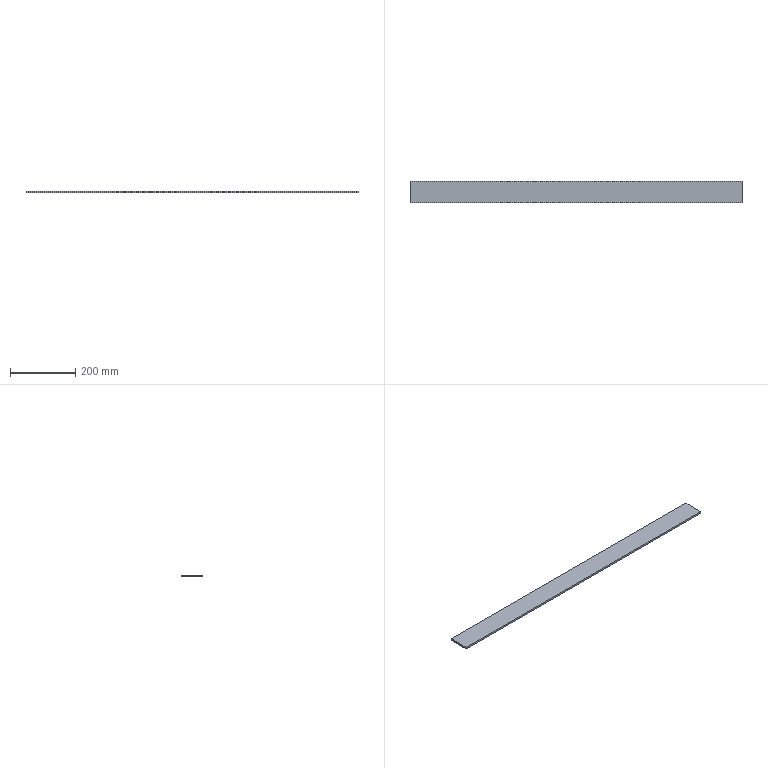Part | STEP file | 04-Support plate | 1 solid | 6 faces | box 1020 x 65 x 6 mm | volume 397800 mm3 | plane 6
STEP:
#1=CARTESIAN_POINT('',(0.,0.,0.));
#2=DIRECTION('',(0.,0.,1.));
#3=DIRECTION('',(1.,0.,0.));
#4=AXIS2_PLACEMENT_3D('',#1,#2,#3);
#5=CARTESIAN_POINT('',(0.,0.,0.));
#6=VERTEX_POINT('',#5);
#7=CARTESIAN_POINT('',(0.,-65.,0.));
#8=VERTEX_POINT('',#7);
#9=CARTESIAN_POINT('',(0.,0.,0.));
#10=DIRECTION('',(0.,-1.,0.));
#11=VECTOR('',#10,1.);
#12=LINE('',#9,#11);
#13=CARTESIAN_POINT('',(0.,0.,6.));
#14=DIRECTION('',(1.,0.,0.));
#15=DIRECTION('',(0.,1.,0.));
#16=AXIS2_PLACEMENT_3D('',#13,#14,#15);
#17=PLANE('',#16);
#18=CARTESIAN_POINT('',(0.,-6.));
#19=DIRECTION('',(-1.,0.));
#20=VECTOR('',#19,1.);
#21=LINE('',#18,#20);
#22=(GEOMETRIC_REPRESENTATION_CONTEXT(2)PARAMETRIC_REPRESENTATION_CONTEXT()REPRESENTATION_CONTEXT('',''));
#23=DEFINITIONAL_REPRESENTATION('',(#21),#22);
#24=PCURVE('',#17,#23);
#25=CARTESIAN_POINT('',(0.,0.,0.));
#26=DIRECTION('',(0.,0.,1.));
#27=DIRECTION('',(1.,0.,0.));
#28=AXIS2_PLACEMENT_3D('',#25,#26,#27);
#29=PLANE('',#28);
#30=CARTESIAN_POINT('',(0.,0.));
#31=DIRECTION('',(0.,-1.));
#32=VECTOR('',#31,1.);
#33=LINE('',#30,#32);
#34=(GEOMETRIC_REPRESENTATION_CONTEXT(2)PARAMETRIC_REPRESENTATION_CONTEXT()REPRESENTATION_CONTEXT('',''));
#35=DEFINITIONAL_REPRESENTATION('',(#33),#34);
#36=PCURVE('',#29,#35);
#37=SURFACE_CURVE('',#12,(#24,#36),.PCURVE_S1.);
#38=EDGE_CURVE('',#6,#8,#37,.T.);
#39=ORIENTED_EDGE('',*,*,#38,.T.);
#40=CARTESIAN_POINT('',(0.,-65.,6.));
#41=VERTEX_POINT('',#40);
#42=CARTESIAN_POINT('',(0.,-65.,6.));
#43=DIRECTION('',(0.,0.,-1.));
#44=VECTOR('',#43,1.);
#45=LINE('',#42,#44);
#46=CARTESIAN_POINT('',(-65.,0.));
#47=DIRECTION('',(0.,-1.));
#48=VECTOR('',#47,1.);
#49=LINE('',#46,#48);
#50=(GEOMETRIC_REPRESENTATION_CONTEXT(2)PARAMETRIC_REPRESENTATION_CONTEXT()REPRESENTATION_CONTEXT('',''));
#51=DEFINITIONAL_REPRESENTATION('',(#49),#50);
#52=PCURVE('',#17,#51);
#53=CARTESIAN_POINT('',(0.,-65.,6.));
#54=DIRECTION('',(0.,1.,0.));
#55=DIRECTION('',(0.,0.,1.));
#56=AXIS2_PLACEMENT_3D('',#53,#54,#55);
#57=PLANE('',#56);
#58=CARTESIAN_POINT('',(0.,0.));
#59=DIRECTION('',(-1.,0.));
#60=VECTOR('',#59,1.);
#61=LINE('',#58,#60);
#62=(GEOMETRIC_REPRESENTATION_CONTEXT(2)PARAMETRIC_REPRESENTATION_CONTEXT()REPRESENTATION_CONTEXT('',''));
#63=DEFINITIONAL_REPRESENTATION('',(#61),#62);
#64=PCURVE('',#57,#63);
#65=SURFACE_CURVE('',#45,(#52,#64),.PCURVE_S1.);
#66=EDGE_CURVE('',#41,#8,#65,.T.);
#67=ORIENTED_EDGE('',*,*,#66,.F.);
#68=CARTESIAN_POINT('',(0.,0.,6.));
#69=VERTEX_POINT('',#68);
#70=CARTESIAN_POINT('',(0.,0.,6.));
#71=DIRECTION('',(0.,-1.,0.));
#72=VECTOR('',#71,1.);
#73=LINE('',#70,#72);
#74=CARTESIAN_POINT('',(0.,0.));
#75=DIRECTION('',(-1.,0.));
#76=VECTOR('',#75,1.);
#77=LINE('',#74,#76);
#78=(GEOMETRIC_REPRESENTATION_CONTEXT(2)PARAMETRIC_REPRESENTATION_CONTEXT()REPRESENTATION_CONTEXT('',''));
#79=DEFINITIONAL_REPRESENTATION('',(#77),#78);
#80=PCURVE('',#17,#79);
#81=CARTESIAN_POINT('',(0.,0.,6.));
#82=DIRECTION('',(0.,0.,1.));
#83=DIRECTION('',(1.,0.,0.));
#84=AXIS2_PLACEMENT_3D('',#81,#82,#83);
#85=PLANE('',#84);
#86=CARTESIAN_POINT('',(0.,0.));
#87=DIRECTION('',(0.,-1.));
#88=VECTOR('',#87,1.);
#89=LINE('',#86,#88);
#90=(GEOMETRIC_REPRESENTATION_CONTEXT(2)PARAMETRIC_REPRESENTATION_CONTEXT()REPRESENTATION_CONTEXT('',''));
#91=DEFINITIONAL_REPRESENTATION('',(#89),#90);
#92=PCURVE('',#85,#91);
#93=SURFACE_CURVE('',#73,(#80,#92),.PCURVE_S1.);
#94=EDGE_CURVE('',#69,#41,#93,.T.);
#95=ORIENTED_EDGE('',*,*,#94,.F.);
#96=CARTESIAN_POINT('',(0.,0.,6.));
#97=DIRECTION('',(0.,0.,-1.));
#98=VECTOR('',#97,1.);
#99=LINE('',#96,#98);
#100=CARTESIAN_POINT('',(0.,0.));
#101=DIRECTION('',(0.,-1.));
#102=VECTOR('',#101,1.);
#103=LINE('',#100,#102);
#104=(GEOMETRIC_REPRESENTATION_CONTEXT(2)PARAMETRIC_REPRESENTATION_CONTEXT()REPRESENTATION_CONTEXT('',''));
#105=DEFINITIONAL_REPRESENTATION('',(#103),#104);
#106=PCURVE('',#17,#105);
#107=CARTESIAN_POINT('',(0.,0.,6.));
#108=DIRECTION('',(0.,-1.,0.));
#109=DIRECTION('',(0.,0.,-1.));
#110=AXIS2_PLACEMENT_3D('',#107,#108,#109);
#111=PLANE('',#110);
#112=CARTESIAN_POINT('',(0.,0.));
#113=DIRECTION('',(1.,0.));
#114=VECTOR('',#113,1.);
#115=LINE('',#112,#114);
#116=(GEOMETRIC_REPRESENTATION_CONTEXT(2)PARAMETRIC_REPRESENTATION_CONTEXT()REPRESENTATION_CONTEXT('',''));
#117=DEFINITIONAL_REPRESENTATION('',(#115),#116);
#118=PCURVE('',#111,#117);
#119=SURFACE_CURVE('',#99,(#106,#118),.PCURVE_S1.);
#120=EDGE_CURVE('',#69,#6,#119,.T.);
#121=ORIENTED_EDGE('',*,*,#120,.T.);
#122=EDGE_LOOP('',(#39,#67,#95,#121));
#123=FACE_BOUND('',#122,.T.);
#124=ADVANCED_FACE('',(#123),#17,.F.);
#125=CARTESIAN_POINT('',(1020.,-65.,0.));
#126=VERTEX_POINT('',#125);
#127=CARTESIAN_POINT('',(0.,-65.,0.));
#128=DIRECTION('',(1.,0.,0.));
#129=VECTOR('',#128,1.);
#130=LINE('',#127,#129);
#131=CARTESIAN_POINT('',(-6.,0.));
#132=DIRECTION('',(0.,1.));
#133=VECTOR('',#132,1.);
#134=LINE('',#131,#133);
#135=(GEOMETRIC_REPRESENTATION_CONTEXT(2)PARAMETRIC_REPRESENTATION_CONTEXT()REPRESENTATION_CONTEXT('',''));
#136=DEFINITIONAL_REPRESENTATION('',(#134),#135);
#137=PCURVE('',#57,#136);
#138=CARTESIAN_POINT('',(0.,-65.));
#139=DIRECTION('',(1.,0.));
#140=VECTOR('',#139,1.);
#141=LINE('',#138,#140);
#142=(GEOMETRIC_REPRESENTATION_CONTEXT(2)PARAMETRIC_REPRESENTATION_CONTEXT()REPRESENTATION_CONTEXT('',''));
#143=DEFINITIONAL_REPRESENTATION('',(#141),#142);
#144=PCURVE('',#29,#143);
#145=SURFACE_CURVE('',#130,(#137,#144),.PCURVE_S1.);
#146=EDGE_CURVE('',#8,#126,#145,.T.);
#147=ORIENTED_EDGE('',*,*,#146,.T.);
#148=CARTESIAN_POINT('',(1020.,-65.,6.));
#149=VERTEX_POINT('',#148);
#150=CARTESIAN_POINT('',(1020.,-65.,6.));
#151=DIRECTION('',(0.,0.,-1.));
#152=VECTOR('',#151,1.);
#153=LINE('',#150,#152);
#154=CARTESIAN_POINT('',(0.,1020.));
#155=DIRECTION('',(-1.,0.));
#156=VECTOR('',#155,1.);
#157=LINE('',#154,#156);
#158=(GEOMETRIC_REPRESENTATION_CONTEXT(2)PARAMETRIC_REPRESENTATION_CONTEXT()REPRESENTATION_CONTEXT('',''));
#159=DEFINITIONAL_REPRESENTATION('',(#157),#158);
#160=PCURVE('',#57,#159);
#161=CARTESIAN_POINT('',(1020.,0.,6.));
#162=DIRECTION('',(-1.,0.,0.));
#163=DIRECTION('',(0.,0.,1.));
#164=AXIS2_PLACEMENT_3D('',#161,#162,#163);
#165=PLANE('',#164);
#166=CARTESIAN_POINT('',(0.,-65.));
#167=DIRECTION('',(-1.,0.));
#168=VECTOR('',#167,1.);
#169=LINE('',#166,#168);
#170=(GEOMETRIC_REPRESENTATION_CONTEXT(2)PARAMETRIC_REPRESENTATION_CONTEXT()REPRESENTATION_CONTEXT('',''));
#171=DEFINITIONAL_REPRESENTATION('',(#169),#170);
#172=PCURVE('',#165,#171);
#173=SURFACE_CURVE('',#153,(#160,#172),.PCURVE_S1.);
#174=EDGE_CURVE('',#149,#126,#173,.T.);
#175=ORIENTED_EDGE('',*,*,#174,.F.);
#176=CARTESIAN_POINT('',(0.,-65.,6.));
#177=DIRECTION('',(1.,0.,0.));
#178=VECTOR('',#177,1.);
#179=LINE('',#176,#178);
#180=CARTESIAN_POINT('',(0.,0.));
#181=DIRECTION('',(0.,1.));
#182=VECTOR('',#181,1.);
#183=LINE('',#180,#182);
#184=(GEOMETRIC_REPRESENTATION_CONTEXT(2)PARAMETRIC_REPRESENTATION_CONTEXT()REPRESENTATION_CONTEXT('',''));
#185=DEFINITIONAL_REPRESENTATION('',(#183),#184);
#186=PCURVE('',#57,#185);
#187=CARTESIAN_POINT('',(0.,-65.));
#188=DIRECTION('',(1.,0.));
#189=VECTOR('',#188,1.);
#190=LINE('',#187,#189);
#191=(GEOMETRIC_REPRESENTATION_CONTEXT(2)PARAMETRIC_REPRESENTATION_CONTEXT()REPRESENTATION_CONTEXT('',''));
#192=DEFINITIONAL_REPRESENTATION('',(#190),#191);
#193=PCURVE('',#85,#192);
#194=SURFACE_CURVE('',#179,(#186,#193),.PCURVE_S1.);
#195=EDGE_CURVE('',#41,#149,#194,.T.);
#196=ORIENTED_EDGE('',*,*,#195,.F.);
#197=ORIENTED_EDGE('',*,*,#66,.T.);
#198=EDGE_LOOP('',(#147,#175,#196,#197));
#199=FACE_BOUND('',#198,.T.);
#200=ADVANCED_FACE('',(#199),#57,.F.);
#201=CARTESIAN_POINT('',(1020.,0.,0.));
#202=VERTEX_POINT('',#201);
#203=CARTESIAN_POINT('',(1020.,0.,0.));
#204=DIRECTION('',(0.,1.,0.));
#205=VECTOR('',#204,1.);
#206=LINE('',#203,#205);
#207=CARTESIAN_POINT('',(-6.,0.));
#208=DIRECTION('',(0.,1.));
#209=VECTOR('',#208,1.);
#210=LINE('',#207,#209);
#211=(GEOMETRIC_REPRESENTATION_CONTEXT(2)PARAMETRIC_REPRESENTATION_CONTEXT()REPRESENTATION_CONTEXT('',''));
#212=DEFINITIONAL_REPRESENTATION('',(#210),#211);
#213=PCURVE('',#165,#212);
#214=CARTESIAN_POINT('',(1020.,0.));
#215=DIRECTION('',(0.,1.));
#216=VECTOR('',#215,1.);
#217=LINE('',#214,#216);
#218=(GEOMETRIC_REPRESENTATION_CONTEXT(2)PARAMETRIC_REPRESENTATION_CONTEXT()REPRESENTATION_CONTEXT('',''));
#219=DEFINITIONAL_REPRESENTATION('',(#217),#218);
#220=PCURVE('',#29,#219);
#221=SURFACE_CURVE('',#206,(#213,#220),.PCURVE_S1.);
#222=EDGE_CURVE('',#126,#202,#221,.T.);
#223=ORIENTED_EDGE('',*,*,#222,.T.);
#224=CARTESIAN_POINT('',(1020.,0.,6.));
#225=VERTEX_POINT('',#224);
#226=CARTESIAN_POINT('',(1020.,0.,6.));
#227=DIRECTION('',(0.,0.,-1.));
#228=VECTOR('',#227,1.);
#229=LINE('',#226,#228);
#230=CARTESIAN_POINT('',(0.,0.));
#231=DIRECTION('',(-1.,0.));
#232=VECTOR('',#231,1.);
#233=LINE('',#230,#232);
#234=(GEOMETRIC_REPRESENTATION_CONTEXT(2)PARAMETRIC_REPRESENTATION_CONTEXT()REPRESENTATION_CONTEXT('',''));
#235=DEFINITIONAL_REPRESENTATION('',(#233),#234);
#236=PCURVE('',#165,#235);
#237=CARTESIAN_POINT('',(0.,1020.));
#238=DIRECTION('',(1.,0.));
#239=VECTOR('',#238,1.);
#240=LINE('',#237,#239);
#241=(GEOMETRIC_REPRESENTATION_CONTEXT(2)PARAMETRIC_REPRESENTATION_CONTEXT()REPRESENTATION_CONTEXT('',''));
#242=DEFINITIONAL_REPRESENTATION('',(#240),#241);
#243=PCURVE('',#111,#242);
#244=SURFACE_CURVE('',#229,(#236,#243),.PCURVE_S1.);
#245=EDGE_CURVE('',#225,#202,#244,.T.);
#246=ORIENTED_EDGE('',*,*,#245,.F.);
#247=CARTESIAN_POINT('',(1020.,0.,6.));
#248=DIRECTION('',(0.,1.,0.));
#249=VECTOR('',#248,1.);
#250=LINE('',#247,#249);
#251=CARTESIAN_POINT('',(0.,0.));
#252=DIRECTION('',(0.,1.));
#253=VECTOR('',#252,1.);
#254=LINE('',#251,#253);
#255=(GEOMETRIC_REPRESENTATION_CONTEXT(2)PARAMETRIC_REPRESENTATION_CONTEXT()REPRESENTATION_CONTEXT('',''));
#256=DEFINITIONAL_REPRESENTATION('',(#254),#255);
#257=PCURVE('',#165,#256);
#258=CARTESIAN_POINT('',(1020.,0.));
#259=DIRECTION('',(0.,1.));
#260=VECTOR('',#259,1.);
#261=LINE('',#258,#260);
#262=(GEOMETRIC_REPRESENTATION_CONTEXT(2)PARAMETRIC_REPRESENTATION_CONTEXT()REPRESENTATION_CONTEXT('',''));
#263=DEFINITIONAL_REPRESENTATION('',(#261),#262);
#264=PCURVE('',#85,#263);
#265=SURFACE_CURVE('',#250,(#257,#264),.PCURVE_S1.);
#266=EDGE_CURVE('',#149,#225,#265,.T.);
#267=ORIENTED_EDGE('',*,*,#266,.F.);
#268=ORIENTED_EDGE('',*,*,#174,.T.);
#269=EDGE_LOOP('',(#223,#246,#267,#268));
#270=FACE_BOUND('',#269,.T.);
#271=ADVANCED_FACE('',(#270),#165,.F.);
#272=CARTESIAN_POINT('',(0.,0.,0.));
#273=DIRECTION('',(-1.,0.,0.));
#274=VECTOR('',#273,1.);
#275=LINE('',#272,#274);
#276=CARTESIAN_POINT('',(6.,0.));
#277=DIRECTION('',(0.,-1.));
#278=VECTOR('',#277,1.);
#279=LINE('',#276,#278);
#280=(GEOMETRIC_REPRESENTATION_CONTEXT(2)PARAMETRIC_REPRESENTATION_CONTEXT()REPRESENTATION_CONTEXT('',''));
#281=DEFINITIONAL_REPRESENTATION('',(#279),#280);
#282=PCURVE('',#111,#281);
#283=CARTESIAN_POINT('',(0.,0.));
#284=DIRECTION('',(-1.,0.));
#285=VECTOR('',#284,1.);
#286=LINE('',#283,#285);
#287=(GEOMETRIC_REPRESENTATION_CONTEXT(2)PARAMETRIC_REPRESENTATION_CONTEXT()REPRESENTATION_CONTEXT('',''));
#288=DEFINITIONAL_REPRESENTATION('',(#286),#287);
#289=PCURVE('',#29,#288);
#290=SURFACE_CURVE('',#275,(#282,#289),.PCURVE_S1.);
#291=EDGE_CURVE('',#202,#6,#290,.T.);
#292=ORIENTED_EDGE('',*,*,#291,.T.);
#293=ORIENTED_EDGE('',*,*,#120,.F.);
#294=CARTESIAN_POINT('',(0.,0.,6.));
#295=DIRECTION('',(-1.,0.,0.));
#296=VECTOR('',#295,1.);
#297=LINE('',#294,#296);
#298=CARTESIAN_POINT('',(0.,0.));
#299=DIRECTION('',(0.,-1.));
#300=VECTOR('',#299,1.);
#301=LINE('',#298,#300);
#302=(GEOMETRIC_REPRESENTATION_CONTEXT(2)PARAMETRIC_REPRESENTATION_CONTEXT()REPRESENTATION_CONTEXT('',''));
#303=DEFINITIONAL_REPRESENTATION('',(#301),#302);
#304=PCURVE('',#111,#303);
#305=CARTESIAN_POINT('',(0.,0.));
#306=DIRECTION('',(-1.,0.));
#307=VECTOR('',#306,1.);
#308=LINE('',#305,#307);
#309=(GEOMETRIC_REPRESENTATION_CONTEXT(2)PARAMETRIC_REPRESENTATION_CONTEXT()REPRESENTATION_CONTEXT('',''));
#310=DEFINITIONAL_REPRESENTATION('',(#308),#309);
#311=PCURVE('',#85,#310);
#312=SURFACE_CURVE('',#297,(#304,#311),.PCURVE_S1.);
#313=EDGE_CURVE('',#225,#69,#312,.T.);
#314=ORIENTED_EDGE('',*,*,#313,.F.);
#315=ORIENTED_EDGE('',*,*,#245,.T.);
#316=EDGE_LOOP('',(#292,#293,#314,#315));
#317=FACE_BOUND('',#316,.T.);
#318=ADVANCED_FACE('',(#317),#111,.F.);
#319=ORIENTED_EDGE('',*,*,#94,.T.);
#320=ORIENTED_EDGE('',*,*,#195,.T.);
#321=ORIENTED_EDGE('',*,*,#266,.T.);
#322=ORIENTED_EDGE('',*,*,#313,.T.);
#323=EDGE_LOOP('',(#319,#320,#321,#322));
#324=FACE_BOUND('',#323,.T.);
#325=ADVANCED_FACE('',(#324),#85,.T.);
#326=ORIENTED_EDGE('',*,*,#38,.F.);
#327=ORIENTED_EDGE('',*,*,#291,.F.);
#328=ORIENTED_EDGE('',*,*,#222,.F.);
#329=ORIENTED_EDGE('',*,*,#146,.F.);
#330=EDGE_LOOP('',(#326,#327,#328,#329));
#331=FACE_BOUND('',#330,.T.);
#332=ADVANCED_FACE('',(#331),#29,.F.);
#333=CLOSED_SHELL('',(#124,#200,#271,#318,#325,#332));
#334=MANIFOLD_SOLID_BREP('',#333);
#335=(LENGTH_UNIT()NAMED_UNIT(*)SI_UNIT(.MILLI.,.METRE.));
#336=UNCERTAINTY_MEASURE_WITH_UNIT(LENGTH_MEASURE(0.0000001),#335,'','');
#337=(NAMED_UNIT(*)PLANE_ANGLE_UNIT()SI_UNIT($,.RADIAN.));
#338=(NAMED_UNIT(*)SI_UNIT($,.STERADIAN.)SOLID_ANGLE_UNIT());
#339=(GEOMETRIC_REPRESENTATION_CONTEXT(3)GLOBAL_UNCERTAINTY_ASSIGNED_CONTEXT((#336))GLOBAL_UNIT_ASSIGNED_CONTEXT((#335,#337,#338))REPRESENTATION_CONTEXT('',''));
#340=ADVANCED_BREP_SHAPE_REPRESENTATION('',(#4,#334),#339);